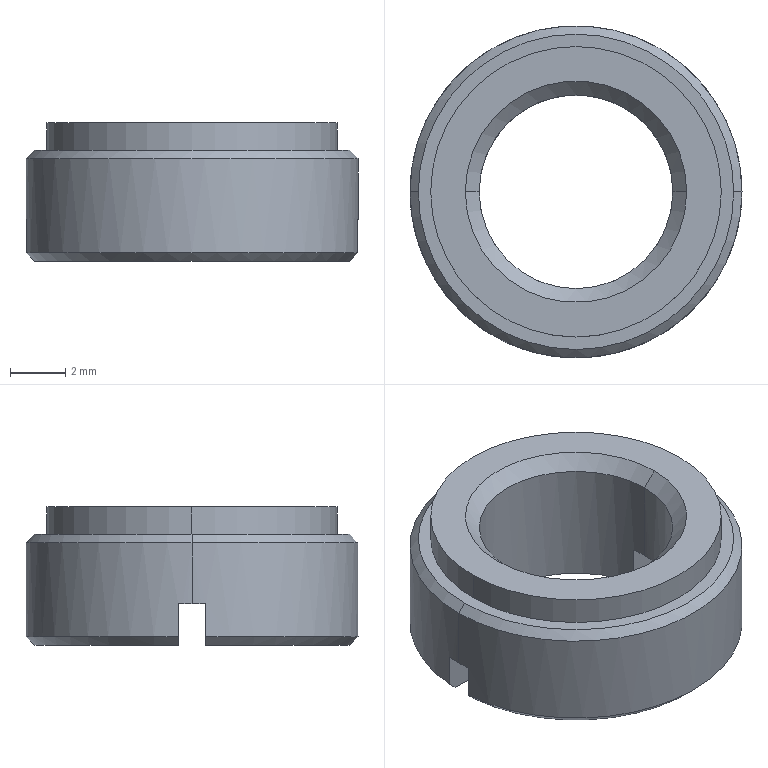Part | SolidWorks | features Chamfer 2, ICE 2, Extrusion 1 | 1 solid | 22 faces | box 12 x 12 x 5 mm | volume 332.916 mm3 | plane 10 | cone 6 | cylinder 6 | commonest cylinder face diameters 7 x2 10.5 x2 12 x2
STEP:
#1=CARTESIAN_POINT('',(5.7,0.,4.));
#2=VERTEX_POINT('',#1);
#3=CARTESIAN_POINT('',(-5.7,0.,4.));
#4=VERTEX_POINT('',#3);
#5=CARTESIAN_POINT('',(0.,0.,4.));
#6=DIRECTION('',(0.,0.,1.));
#7=DIRECTION('',(1.,0.,0.));
#8=AXIS2_PLACEMENT_3D('',#5,#6,#7);
#9=CIRCLE('',#8,5.7);
#10=EDGE_CURVE('',#2,#4,#9,.T.);
#11=ORIENTED_EDGE('',*,*,#10,.F.);
#12=CARTESIAN_POINT('',(6.,0.,3.7));
#13=VERTEX_POINT('',#12);
#14=CARTESIAN_POINT('',(5.7,0.,4.));
#15=DIRECTION('',(0.7071,0.,-0.7071));
#16=VECTOR('',#15,1000.);
#17=LINE('',#14,#16);
#18=EDGE_CURVE('',#2,#13,#17,.T.);
#19=ORIENTED_EDGE('',*,*,#18,.T.);
#20=CARTESIAN_POINT('',(-6.,0.,3.7));
#21=VERTEX_POINT('',#20);
#22=CARTESIAN_POINT('',(0.,0.,3.7));
#23=DIRECTION('',(0.,0.,-1.));
#24=DIRECTION('',(1.,0.,0.));
#25=AXIS2_PLACEMENT_3D('',#22,#23,#24);
#26=CIRCLE('',#25,6.);
#27=EDGE_CURVE('',#21,#13,#26,.T.);
#28=ORIENTED_EDGE('',*,*,#27,.F.);
#29=CARTESIAN_POINT('',(-5.7,0.,4.));
#30=DIRECTION('',(-0.7071,0.,-0.7071));
#31=VECTOR('',#30,1000.);
#32=LINE('',#29,#31);
#33=EDGE_CURVE('',#4,#21,#32,.T.);
#34=ORIENTED_EDGE('',*,*,#33,.F.);
#35=EDGE_LOOP('',(#11,#19,#28,#34));
#36=FACE_OUTER_BOUND('',#35,.T.);
#37=CARTESIAN_POINT('',(0.,0.,4.));
#38=DIRECTION('',(0.,0.,-1.));
#39=DIRECTION('',(-1.,0.,0.));
#40=AXIS2_PLACEMENT_3D('',#37,#38,#39);
#41=CONICAL_SURFACE('',#40,5.7,0.7854);
#42=ADVANCED_FACE('',(#36),#41,.T.);
#43=CARTESIAN_POINT('',(5.25,0.,4.));
#44=VERTEX_POINT('',#43);
#45=CARTESIAN_POINT('',(-5.25,0.,4.));
#46=VERTEX_POINT('',#45);
#47=CARTESIAN_POINT('',(0.,0.,4.));
#48=DIRECTION('',(0.,0.,1.));
#49=DIRECTION('',(1.,0.,0.));
#50=AXIS2_PLACEMENT_3D('',#47,#48,#49);
#51=CIRCLE('',#50,5.25);
#52=EDGE_CURVE('',#44,#46,#51,.T.);
#53=ORIENTED_EDGE('',*,*,#52,.T.);
#54=CARTESIAN_POINT('',(-5.25,0.,5.));
#55=VERTEX_POINT('',#54);
#56=CARTESIAN_POINT('',(-5.25,0.,4.));
#57=DIRECTION('',(0.,0.,1.));
#58=VECTOR('',#57,1000.);
#59=LINE('',#56,#58);
#60=EDGE_CURVE('',#46,#55,#59,.T.);
#61=ORIENTED_EDGE('',*,*,#60,.T.);
#62=CARTESIAN_POINT('',(5.25,0.,5.));
#63=VERTEX_POINT('',#62);
#64=CARTESIAN_POINT('',(0.,0.,5.));
#65=DIRECTION('',(0.,0.,1.));
#66=DIRECTION('',(1.,0.,0.));
#67=AXIS2_PLACEMENT_3D('',#64,#65,#66);
#68=CIRCLE('',#67,5.25);
#69=EDGE_CURVE('',#63,#55,#68,.T.);
#70=ORIENTED_EDGE('',*,*,#69,.F.);
#71=CARTESIAN_POINT('',(5.25,0.,4.));
#72=DIRECTION('',(0.,0.,1.));
#73=VECTOR('',#72,1000.);
#74=LINE('',#71,#73);
#75=EDGE_CURVE('',#44,#63,#74,.T.);
#76=ORIENTED_EDGE('',*,*,#75,.F.);
#77=EDGE_LOOP('',(#53,#61,#70,#76));
#78=FACE_OUTER_BOUND('',#77,.T.);
#79=CARTESIAN_POINT('',(0.,0.,4.));
#80=DIRECTION('',(0.,0.,1.));
#81=DIRECTION('',(1.,0.,0.));
#82=AXIS2_PLACEMENT_3D('',#79,#80,#81);
#83=CYLINDRICAL_SURFACE('',#82,5.25);
#84=ADVANCED_FACE('',(#78),#83,.T.);
#85=CARTESIAN_POINT('',(-3.5,0.,4.5));
#86=VERTEX_POINT('',#85);
#87=CARTESIAN_POINT('',(3.5,0.,4.5));
#88=VERTEX_POINT('',#87);
#89=CARTESIAN_POINT('',(0.,0.,4.5));
#90=DIRECTION('',(0.,0.,1.));
#91=DIRECTION('',(1.,0.,0.));
#92=AXIS2_PLACEMENT_3D('',#89,#90,#91);
#93=CIRCLE('',#92,3.5);
#94=EDGE_CURVE('',#86,#88,#93,.T.);
#95=ORIENTED_EDGE('',*,*,#94,.F.);
#96=CARTESIAN_POINT('',(-4.,0.,5.));
#97=VERTEX_POINT('',#96);
#98=CARTESIAN_POINT('',(-3.5,0.,4.5));
#99=DIRECTION('',(-0.7071,0.,0.7071));
#100=VECTOR('',#99,1000.);
#101=LINE('',#98,#100);
#102=EDGE_CURVE('',#86,#97,#101,.T.);
#103=ORIENTED_EDGE('',*,*,#102,.T.);
#104=CARTESIAN_POINT('',(4.,0.,5.));
#105=VERTEX_POINT('',#104);
#106=CARTESIAN_POINT('',(0.,0.,5.));
#107=DIRECTION('',(0.,0.,-1.));
#108=DIRECTION('',(1.,0.,0.));
#109=AXIS2_PLACEMENT_3D('',#106,#107,#108);
#110=CIRCLE('',#109,4.);
#111=EDGE_CURVE('',#105,#97,#110,.T.);
#112=ORIENTED_EDGE('',*,*,#111,.F.);
#113=CARTESIAN_POINT('',(3.5,0.,4.5));
#114=DIRECTION('',(0.7071,0.,0.7071));
#115=VECTOR('',#114,1000.);
#116=LINE('',#113,#115);
#117=EDGE_CURVE('',#88,#105,#116,.T.);
#118=ORIENTED_EDGE('',*,*,#117,.F.);
#119=EDGE_LOOP('',(#95,#103,#112,#118));
#120=FACE_OUTER_BOUND('',#119,.T.);
#121=CARTESIAN_POINT('',(0.,0.,4.5));
#122=DIRECTION('',(0.,0.,1.));
#123=DIRECTION('',(1.,0.,0.));
#124=AXIS2_PLACEMENT_3D('',#121,#122,#123);
#125=CONICAL_SURFACE('',#124,3.5,0.7854);
#126=ADVANCED_FACE('',(#120),#125,.F.);
#127=ORIENTED_EDGE('',*,*,#94,.T.);
#128=CARTESIAN_POINT('',(3.5,0.,1.5));
#129=VERTEX_POINT('',#128);
#130=CARTESIAN_POINT('',(3.5,0.,5.));
#131=DIRECTION('',(0.,0.,-1.));
#132=VECTOR('',#131,1000.);
#133=LINE('',#130,#132);
#134=EDGE_CURVE('',#88,#129,#133,.T.);
#135=ORIENTED_EDGE('',*,*,#134,.T.);
#136=CARTESIAN_POINT('',(3.464,-0.5,1.5));
#137=VERTEX_POINT('',#136);
#138=CARTESIAN_POINT('',(0.,0.,1.5));
#139=DIRECTION('',(0.,0.,-1.));
#140=DIRECTION('',(-1.,0.,0.));
#141=AXIS2_PLACEMENT_3D('',#138,#139,#140);
#142=CIRCLE('',#141,3.5);
#143=EDGE_CURVE('',#129,#137,#142,.T.);
#144=ORIENTED_EDGE('',*,*,#143,.T.);
#145=CARTESIAN_POINT('',(3.464,-0.5,0.));
#146=VERTEX_POINT('',#145);
#147=CARTESIAN_POINT('',(3.464,-0.5,5.));
#148=DIRECTION('',(0.,0.,1.));
#149=VECTOR('',#148,1000.);
#150=LINE('',#147,#149);
#151=EDGE_CURVE('',#146,#137,#150,.T.);
#152=ORIENTED_EDGE('',*,*,#151,.F.);
#153=CARTESIAN_POINT('',(-3.464,-0.5,0.));
#154=VERTEX_POINT('',#153);
#155=CARTESIAN_POINT('',(0.,0.,0.));
#156=DIRECTION('',(0.,0.,1.));
#157=DIRECTION('',(1.,0.,0.));
#158=AXIS2_PLACEMENT_3D('',#155,#156,#157);
#159=CIRCLE('',#158,3.5);
#160=EDGE_CURVE('',#154,#146,#159,.T.);
#161=ORIENTED_EDGE('',*,*,#160,.F.);
#162=CARTESIAN_POINT('',(-3.464,-0.5,1.5));
#163=VERTEX_POINT('',#162);
#164=CARTESIAN_POINT('',(-3.464,-0.5,5.));
#165=DIRECTION('',(0.,0.,-1.));
#166=VECTOR('',#165,1000.);
#167=LINE('',#164,#166);
#168=EDGE_CURVE('',#163,#154,#167,.T.);
#169=ORIENTED_EDGE('',*,*,#168,.F.);
#170=CARTESIAN_POINT('',(-3.5,0.,1.5));
#171=VERTEX_POINT('',#170);
#172=CARTESIAN_POINT('',(0.,0.,1.5));
#173=DIRECTION('',(0.,0.,-1.));
#174=DIRECTION('',(-1.,0.,0.));
#175=AXIS2_PLACEMENT_3D('',#172,#173,#174);
#176=CIRCLE('',#175,3.5);
#177=EDGE_CURVE('',#163,#171,#176,.T.);
#178=ORIENTED_EDGE('',*,*,#177,.T.);
#179=CARTESIAN_POINT('',(-3.5,0.,5.));
#180=DIRECTION('',(0.,0.,-1.));
#181=VECTOR('',#180,1000.);
#182=LINE('',#179,#181);
#183=EDGE_CURVE('',#86,#171,#182,.T.);
#184=ORIENTED_EDGE('',*,*,#183,.F.);
#185=EDGE_LOOP('',(#127,#135,#144,#152,#161,#169,#178,#184));
#186=FACE_OUTER_BOUND('',#185,.T.);
#187=CARTESIAN_POINT('',(0.,0.,5.));
#188=DIRECTION('',(0.,0.,-1.));
#189=DIRECTION('',(-1.,0.,0.));
#190=AXIS2_PLACEMENT_3D('',#187,#188,#189);
#191=CYLINDRICAL_SURFACE('',#190,3.5);
#192=ADVANCED_FACE('',(#186),#191,.F.);
#193=ORIENTED_EDGE('',*,*,#27,.T.);
#194=CARTESIAN_POINT('',(6.,0.,1.5));
#195=VERTEX_POINT('',#194);
#196=CARTESIAN_POINT('',(6.,0.,5.));
#197=DIRECTION('',(0.,0.,-1.));
#198=VECTOR('',#197,1000.);
#199=LINE('',#196,#198);
#200=EDGE_CURVE('',#13,#195,#199,.T.);
#201=ORIENTED_EDGE('',*,*,#200,.T.);
#202=CARTESIAN_POINT('',(5.979,0.5,1.5));
#203=VERTEX_POINT('',#202);
#204=CARTESIAN_POINT('',(0.,0.,1.5));
#205=DIRECTION('',(0.,0.,-1.));
#206=DIRECTION('',(-1.,0.,0.));
#207=AXIS2_PLACEMENT_3D('',#204,#205,#206);
#208=CIRCLE('',#207,6.);
#209=EDGE_CURVE('',#203,#195,#208,.T.);
#210=ORIENTED_EDGE('',*,*,#209,.F.);
#211=CARTESIAN_POINT('',(5.979,0.5,0.3));
#212=VERTEX_POINT('',#211);
#213=CARTESIAN_POINT('',(5.979,0.5,5.));
#214=DIRECTION('',(0.,0.,-1.));
#215=VECTOR('',#214,1000.);
#216=LINE('',#213,#215);
#217=EDGE_CURVE('',#203,#212,#216,.T.);
#218=ORIENTED_EDGE('',*,*,#217,.T.);
#219=CARTESIAN_POINT('',(-5.979,0.5,0.3));
#220=VERTEX_POINT('',#219);
#221=CARTESIAN_POINT('',(0.,0.,0.3));
#222=DIRECTION('',(0.,0.,1.));
#223=DIRECTION('',(1.,0.,0.));
#224=AXIS2_PLACEMENT_3D('',#221,#222,#223);
#225=CIRCLE('',#224,6.);
#226=EDGE_CURVE('',#212,#220,#225,.T.);
#227=ORIENTED_EDGE('',*,*,#226,.T.);
#228=CARTESIAN_POINT('',(-5.979,0.5,1.5));
#229=VERTEX_POINT('',#228);
#230=CARTESIAN_POINT('',(-5.979,0.5,5.));
#231=DIRECTION('',(0.,0.,1.));
#232=VECTOR('',#231,1000.);
#233=LINE('',#230,#232);
#234=EDGE_CURVE('',#220,#229,#233,.T.);
#235=ORIENTED_EDGE('',*,*,#234,.T.);
#236=CARTESIAN_POINT('',(-6.,0.,1.5));
#237=VERTEX_POINT('',#236);
#238=CARTESIAN_POINT('',(0.,0.,1.5));
#239=DIRECTION('',(0.,0.,-1.));
#240=DIRECTION('',(-1.,0.,0.));
#241=AXIS2_PLACEMENT_3D('',#238,#239,#240);
#242=CIRCLE('',#241,6.);
#243=EDGE_CURVE('',#237,#229,#242,.T.);
#244=ORIENTED_EDGE('',*,*,#243,.F.);
#245=CARTESIAN_POINT('',(-6.,0.,5.));
#246=DIRECTION('',(0.,0.,-1.));
#247=VECTOR('',#246,1000.);
#248=LINE('',#245,#247);
#249=EDGE_CURVE('',#21,#237,#248,.T.);
#250=ORIENTED_EDGE('',*,*,#249,.F.);
#251=EDGE_LOOP('',(#193,#201,#210,#218,#227,#235,#244,#250));
#252=FACE_OUTER_BOUND('',#251,.T.);
#253=CARTESIAN_POINT('',(0.,0.,5.));
#254=DIRECTION('',(0.,0.,-1.));
#255=DIRECTION('',(-1.,0.,0.));
#256=AXIS2_PLACEMENT_3D('',#253,#254,#255);
#257=CYLINDRICAL_SURFACE('',#256,6.);
#258=ADVANCED_FACE('',(#252),#257,.T.);
#259=ORIENTED_EDGE('',*,*,#111,.T.);
#260=CARTESIAN_POINT('',(0.,0.,5.));
#261=DIRECTION('',(0.,0.,-1.));
#262=DIRECTION('',(1.,0.,0.));
#263=AXIS2_PLACEMENT_3D('',#260,#261,#262);
#264=CIRCLE('',#263,4.);
#265=EDGE_CURVE('',#97,#105,#264,.T.);
#266=ORIENTED_EDGE('',*,*,#265,.T.);
#267=EDGE_LOOP('',(#259,#266));
#268=FACE_BOUND('',#267,.T.);
#269=ORIENTED_EDGE('',*,*,#69,.T.);
#270=CARTESIAN_POINT('',(0.,0.,5.));
#271=DIRECTION('',(0.,0.,1.));
#272=DIRECTION('',(1.,0.,0.));
#273=AXIS2_PLACEMENT_3D('',#270,#271,#272);
#274=CIRCLE('',#273,5.25);
#275=EDGE_CURVE('',#55,#63,#274,.T.);
#276=ORIENTED_EDGE('',*,*,#275,.T.);
#277=EDGE_LOOP('',(#269,#276));
#278=FACE_OUTER_BOUND('',#277,.T.);
#279=CARTESIAN_POINT('',(0.,0.,5.));
#280=DIRECTION('',(0.,0.,1.));
#281=DIRECTION('',(1.,0.,0.));
#282=AXIS2_PLACEMENT_3D('',#279,#280,#281);
#283=PLANE('',#282);
#284=ADVANCED_FACE('',(#268,#278),#283,.T.);
#285=ORIENTED_EDGE('',*,*,#200,.F.);
#286=CARTESIAN_POINT('',(0.,0.,3.7));
#287=DIRECTION('',(0.,0.,-1.));
#288=DIRECTION('',(1.,0.,0.));
#289=AXIS2_PLACEMENT_3D('',#286,#287,#288);
#290=CIRCLE('',#289,6.);
#291=EDGE_CURVE('',#13,#21,#290,.T.);
#292=ORIENTED_EDGE('',*,*,#291,.T.);
#293=ORIENTED_EDGE('',*,*,#249,.T.);
#294=CARTESIAN_POINT('',(-5.979,-0.5,1.5));
#295=VERTEX_POINT('',#294);
#296=CARTESIAN_POINT('',(0.,0.,1.5));
#297=DIRECTION('',(0.,0.,-1.));
#298=DIRECTION('',(-1.,0.,0.));
#299=AXIS2_PLACEMENT_3D('',#296,#297,#298);
#300=CIRCLE('',#299,6.);
#301=EDGE_CURVE('',#295,#237,#300,.T.);
#302=ORIENTED_EDGE('',*,*,#301,.F.);
#303=CARTESIAN_POINT('',(-5.979,-0.5,0.3));
#304=VERTEX_POINT('',#303);
#305=CARTESIAN_POINT('',(-5.979,-0.5,5.));
#306=DIRECTION('',(0.,0.,-1.));
#307=VECTOR('',#306,1000.);
#308=LINE('',#305,#307);
#309=EDGE_CURVE('',#295,#304,#308,.T.);
#310=ORIENTED_EDGE('',*,*,#309,.T.);
#311=CARTESIAN_POINT('',(5.979,-0.5,0.3));
#312=VERTEX_POINT('',#311);
#313=CARTESIAN_POINT('',(0.,0.,0.3));
#314=DIRECTION('',(0.,0.,1.));
#315=DIRECTION('',(1.,0.,0.));
#316=AXIS2_PLACEMENT_3D('',#313,#314,#315);
#317=CIRCLE('',#316,6.);
#318=EDGE_CURVE('',#304,#312,#317,.T.);
#319=ORIENTED_EDGE('',*,*,#318,.T.);
#320=CARTESIAN_POINT('',(5.979,-0.5,1.5));
#321=VERTEX_POINT('',#320);
#322=CARTESIAN_POINT('',(5.979,-0.5,5.));
#323=DIRECTION('',(0.,0.,1.));
#324=VECTOR('',#323,1000.);
#325=LINE('',#322,#324);
#326=EDGE_CURVE('',#312,#321,#325,.T.);
#327=ORIENTED_EDGE('',*,*,#326,.T.);
#328=CARTESIAN_POINT('',(0.,0.,1.5));
#329=DIRECTION('',(0.,0.,-1.));
#330=DIRECTION('',(-1.,0.,0.));
#331=AXIS2_PLACEMENT_3D('',#328,#329,#330);
#332=CIRCLE('',#331,6.);
#333=EDGE_CURVE('',#195,#321,#332,.T.);
#334=ORIENTED_EDGE('',*,*,#333,.F.);
#335=EDGE_LOOP('',(#285,#292,#293,#302,#310,#319,#327,#334));
#336=FACE_OUTER_BOUND('',#335,.T.);
#337=CARTESIAN_POINT('',(0.,0.,5.));
#338=DIRECTION('',(0.,0.,-1.));
#339=DIRECTION('',(-1.,0.,0.));
#340=AXIS2_PLACEMENT_3D('',#337,#338,#339);
#341=CYLINDRICAL_SURFACE('',#340,6.);
#342=ADVANCED_FACE('',(#336),#341,.T.);
#343=CARTESIAN_POINT('',(-5.678,0.5,0.));
#344=VERTEX_POINT('',#343);
#345=CARTESIAN_POINT('',(-3.464,0.5,0.));
#346=VERTEX_POINT('',#345);
#347=CARTESIAN_POINT('',(8.749,0.5,0.));
#348=DIRECTION('',(1.,0.,0.));
#349=VECTOR('',#348,1000.);
#350=LINE('',#347,#349);
#351=EDGE_CURVE('',#344,#346,#350,.T.);
#352=ORIENTED_EDGE('',*,*,#351,.F.);
#353=CARTESIAN_POINT('',(5.678,0.5,0.));
#354=VERTEX_POINT('',#353);
#355=CARTESIAN_POINT('',(0.,0.,0.));
#356=DIRECTION('',(0.,0.,-1.));
#357=DIRECTION('',(1.,0.,0.));
#358=AXIS2_PLACEMENT_3D('',#355,#356,#357);
#359=CIRCLE('',#358,5.7);
#360=EDGE_CURVE('',#344,#354,#359,.T.);
#361=ORIENTED_EDGE('',*,*,#360,.T.);
#362=CARTESIAN_POINT('',(3.464,0.5,0.));
#363=VERTEX_POINT('',#362);
#364=CARTESIAN_POINT('',(8.749,0.5,0.));
#365=DIRECTION('',(1.,0.,0.));
#366=VECTOR('',#365,1000.);
#367=LINE('',#364,#366);
#368=EDGE_CURVE('',#363,#354,#367,.T.);
#369=ORIENTED_EDGE('',*,*,#368,.F.);
#370=CARTESIAN_POINT('',(0.,0.,0.));
#371=DIRECTION('',(0.,0.,1.));
#372=DIRECTION('',(1.,0.,0.));
#373=AXIS2_PLACEMENT_3D('',#370,#371,#372);
#374=CIRCLE('',#373,3.5);
#375=EDGE_CURVE('',#363,#346,#374,.T.);
#376=ORIENTED_EDGE('',*,*,#375,.T.);
#377=EDGE_LOOP('',(#352,#361,#369,#376));
#378=FACE_OUTER_BOUND('',#377,.T.);
#379=CARTESIAN_POINT('',(0.,0.,0.));
#380=DIRECTION('',(0.,0.,1.));
#381=DIRECTION('',(1.,0.,0.));
#382=AXIS2_PLACEMENT_3D('',#379,#380,#381);
#383=PLANE('',#382);
#384=ADVANCED_FACE('',(#378),#383,.F.);
#385=CARTESIAN_POINT('',(5.678,-0.5,0.));
#386=VERTEX_POINT('',#385);
#387=CARTESIAN_POINT('',(8.749,-0.5,0.));
#388=DIRECTION('',(-1.,0.,0.));
#389=VECTOR('',#388,1000.);
#390=LINE('',#387,#389);
#391=EDGE_CURVE('',#386,#146,#390,.T.);
#392=ORIENTED_EDGE('',*,*,#391,.F.);
#393=CARTESIAN_POINT('',(-5.678,-0.5,0.));
#394=VERTEX_POINT('',#393);
#395=CARTESIAN_POINT('',(0.,0.,0.));
#396=DIRECTION('',(0.,0.,-1.));
#397=DIRECTION('',(1.,0.,0.));
#398=AXIS2_PLACEMENT_3D('',#395,#396,#397);
#399=CIRCLE('',#398,5.7);
#400=EDGE_CURVE('',#386,#394,#399,.T.);
#401=ORIENTED_EDGE('',*,*,#400,.T.);
#402=CARTESIAN_POINT('',(8.749,-0.5,0.));
#403=DIRECTION('',(-1.,0.,0.));
#404=VECTOR('',#403,1000.);
#405=LINE('',#402,#404);
#406=EDGE_CURVE('',#154,#394,#405,.T.);
#407=ORIENTED_EDGE('',*,*,#406,.F.);
#408=ORIENTED_EDGE('',*,*,#160,.T.);
#409=EDGE_LOOP('',(#392,#401,#407,#408));
#410=FACE_OUTER_BOUND('',#409,.T.);
#411=CARTESIAN_POINT('',(0.,0.,0.));
#412=DIRECTION('',(0.,0.,1.));
#413=DIRECTION('',(1.,0.,0.));
#414=AXIS2_PLACEMENT_3D('',#411,#412,#413);
#415=PLANE('',#414);
#416=ADVANCED_FACE('',(#410),#415,.F.);
#417=ORIENTED_EDGE('',*,*,#134,.F.);
#418=CARTESIAN_POINT('',(0.,0.,4.5));
#419=DIRECTION('',(0.,0.,1.));
#420=DIRECTION('',(1.,0.,0.));
#421=AXIS2_PLACEMENT_3D('',#418,#419,#420);
#422=CIRCLE('',#421,3.5);
#423=EDGE_CURVE('',#88,#86,#422,.T.);
#424=ORIENTED_EDGE('',*,*,#423,.T.);
#425=ORIENTED_EDGE('',*,*,#183,.T.);
#426=CARTESIAN_POINT('',(-3.464,0.5,1.5));
#427=VERTEX_POINT('',#426);
#428=CARTESIAN_POINT('',(0.,0.,1.5));
#429=DIRECTION('',(0.,0.,-1.));
#430=DIRECTION('',(-1.,0.,0.));
#431=AXIS2_PLACEMENT_3D('',#428,#429,#430);
#432=CIRCLE('',#431,3.5);
#433=EDGE_CURVE('',#171,#427,#432,.T.);
#434=ORIENTED_EDGE('',*,*,#433,.T.);
#435=CARTESIAN_POINT('',(-3.464,0.5,5.));
#436=DIRECTION('',(0.,0.,1.));
#437=VECTOR('',#436,1000.);
#438=LINE('',#435,#437);
#439=EDGE_CURVE('',#346,#427,#438,.T.);
#440=ORIENTED_EDGE('',*,*,#439,.F.);
#441=ORIENTED_EDGE('',*,*,#375,.F.);
#442=CARTESIAN_POINT('',(3.464,0.5,1.5));
#443=VERTEX_POINT('',#442);
#444=CARTESIAN_POINT('',(3.464,0.5,5.));
#445=DIRECTION('',(0.,0.,-1.));
#446=VECTOR('',#445,1000.);
#447=LINE('',#444,#446);
#448=EDGE_CURVE('',#443,#363,#447,.T.);
#449=ORIENTED_EDGE('',*,*,#448,.F.);
#450=CARTESIAN_POINT('',(0.,0.,1.5));
#451=DIRECTION('',(0.,0.,-1.));
#452=DIRECTION('',(-1.,0.,0.));
#453=AXIS2_PLACEMENT_3D('',#450,#451,#452);
#454=CIRCLE('',#453,3.5);
#455=EDGE_CURVE('',#443,#129,#454,.T.);
#456=ORIENTED_EDGE('',*,*,#455,.T.);
#457=EDGE_LOOP('',(#417,#424,#425,#434,#440,#441,#449,#456));
#458=FACE_OUTER_BOUND('',#457,.T.);
#459=CARTESIAN_POINT('',(0.,0.,5.));
#460=DIRECTION('',(0.,0.,-1.));
#461=DIRECTION('',(-1.,0.,0.));
#462=AXIS2_PLACEMENT_3D('',#459,#460,#461);
#463=CYLINDRICAL_SURFACE('',#462,3.5);
#464=ADVANCED_FACE('',(#458),#463,.F.);
#465=ORIENTED_EDGE('',*,*,#102,.F.);
#466=ORIENTED_EDGE('',*,*,#423,.F.);
#467=ORIENTED_EDGE('',*,*,#117,.T.);
#468=ORIENTED_EDGE('',*,*,#265,.F.);
#469=EDGE_LOOP('',(#465,#466,#467,#468));
#470=FACE_OUTER_BOUND('',#469,.T.);
#471=CARTESIAN_POINT('',(0.,0.,4.5));
#472=DIRECTION('',(0.,0.,1.));
#473=DIRECTION('',(1.,0.,0.));
#474=AXIS2_PLACEMENT_3D('',#471,#472,#473);
#475=CONICAL_SURFACE('',#474,3.5,0.7854);
#476=ADVANCED_FACE('',(#470),#475,.F.);
#477=ORIENTED_EDGE('',*,*,#301,.T.);
#478=ORIENTED_EDGE('',*,*,#243,.T.);
#479=CARTESIAN_POINT('',(8.749,0.5,1.5));
#480=DIRECTION('',(1.,0.,0.));
#481=VECTOR('',#480,1000.);
#482=LINE('',#479,#481);
#483=EDGE_CURVE('',#229,#427,#482,.T.);
#484=ORIENTED_EDGE('',*,*,#483,.T.);
#485=ORIENTED_EDGE('',*,*,#433,.F.);
#486=ORIENTED_EDGE('',*,*,#177,.F.);
#487=CARTESIAN_POINT('',(8.749,-0.5,1.5));
#488=DIRECTION('',(-1.,0.,0.));
#489=VECTOR('',#488,1000.);
#490=LINE('',#487,#489);
#491=EDGE_CURVE('',#163,#295,#490,.T.);
#492=ORIENTED_EDGE('',*,*,#491,.T.);
#493=EDGE_LOOP('',(#477,#478,#484,#485,#486,#492));
#494=FACE_OUTER_BOUND('',#493,.T.);
#495=CARTESIAN_POINT('',(8.749,-0.5,1.5));
#496=DIRECTION('',(0.,0.,-1.));
#497=DIRECTION('',(-1.,0.,0.));
#498=AXIS2_PLACEMENT_3D('',#495,#496,#497);
#499=PLANE('',#498);
#500=ADVANCED_FACE('',(#494),#499,.T.);
#501=ORIENTED_EDGE('',*,*,#406,.T.);
#502=CARTESIAN_POINT('',(-5.678,-0.5,0.));
#503=CARTESIAN_POINT('',(-5.778,-0.5,0.09999));
#504=CARTESIAN_POINT('',(-5.879,-0.5,0.2));
#505=CARTESIAN_POINT('',(-5.979,-0.5,0.3));
#506=B_SPLINE_CURVE_WITH_KNOTS('',3,(#502,#503,#504,#505),.UNSPECIFIED.,.F.,.F.,(4,4),(0.,0.000425),.UNSPECIFIED.);
#507=EDGE_CURVE('',#394,#304,#506,.T.);
#508=ORIENTED_EDGE('',*,*,#507,.T.);
#509=ORIENTED_EDGE('',*,*,#309,.F.);
#510=ORIENTED_EDGE('',*,*,#491,.F.);
#511=ORIENTED_EDGE('',*,*,#168,.T.);
#512=EDGE_LOOP('',(#501,#508,#509,#510,#511));
#513=FACE_OUTER_BOUND('',#512,.T.);
#514=CARTESIAN_POINT('',(8.749,-0.5,1.5));
#515=DIRECTION('',(0.,-1.,0.));
#516=DIRECTION('',(0.,0.,-1.));
#517=AXIS2_PLACEMENT_3D('',#514,#515,#516);
#518=PLANE('',#517);
#519=ADVANCED_FACE('',(#513),#518,.F.);
#520=ORIENTED_EDGE('',*,*,#234,.F.);
#521=CARTESIAN_POINT('',(-5.979,0.5,0.3));
#522=CARTESIAN_POINT('',(-5.879,0.5,0.2));
#523=CARTESIAN_POINT('',(-5.778,0.5,0.09999));
#524=CARTESIAN_POINT('',(-5.678,0.5,0.));
#525=B_SPLINE_CURVE_WITH_KNOTS('',3,(#521,#522,#523,#524),.UNSPECIFIED.,.F.,.F.,(4,4),(0.,0.000425),.UNSPECIFIED.);
#526=EDGE_CURVE('',#220,#344,#525,.T.);
#527=ORIENTED_EDGE('',*,*,#526,.T.);
#528=ORIENTED_EDGE('',*,*,#351,.T.);
#529=ORIENTED_EDGE('',*,*,#439,.T.);
#530=ORIENTED_EDGE('',*,*,#483,.F.);
#531=EDGE_LOOP('',(#520,#527,#528,#529,#530));
#532=FACE_OUTER_BOUND('',#531,.T.);
#533=CARTESIAN_POINT('',(8.749,0.5,1.5));
#534=DIRECTION('',(0.,1.,0.));
#535=DIRECTION('',(0.,0.,1.));
#536=AXIS2_PLACEMENT_3D('',#533,#534,#535);
#537=PLANE('',#536);
#538=ADVANCED_FACE('',(#532),#537,.F.);
#539=ORIENTED_EDGE('',*,*,#368,.T.);
#540=CARTESIAN_POINT('',(5.678,0.5,0.));
#541=CARTESIAN_POINT('',(5.778,0.5,0.09999));
#542=CARTESIAN_POINT('',(5.879,0.5,0.2));
#543=CARTESIAN_POINT('',(5.979,0.5,0.3));
#544=B_SPLINE_CURVE_WITH_KNOTS('',3,(#540,#541,#542,#543),.UNSPECIFIED.,.F.,.F.,(4,4),(0.,0.000425),.UNSPECIFIED.);
#545=EDGE_CURVE('',#354,#212,#544,.T.);
#546=ORIENTED_EDGE('',*,*,#545,.T.);
#547=ORIENTED_EDGE('',*,*,#217,.F.);
#548=CARTESIAN_POINT('',(8.749,0.5,1.5));
#549=DIRECTION('',(1.,0.,0.));
#550=VECTOR('',#549,1000.);
#551=LINE('',#548,#550);
#552=EDGE_CURVE('',#443,#203,#551,.T.);
#553=ORIENTED_EDGE('',*,*,#552,.F.);
#554=ORIENTED_EDGE('',*,*,#448,.T.);
#555=EDGE_LOOP('',(#539,#546,#547,#553,#554));
#556=FACE_OUTER_BOUND('',#555,.T.);
#557=CARTESIAN_POINT('',(8.749,0.5,1.5));
#558=DIRECTION('',(0.,1.,0.));
#559=DIRECTION('',(0.,0.,1.));
#560=AXIS2_PLACEMENT_3D('',#557,#558,#559);
#561=PLANE('',#560);
#562=ADVANCED_FACE('',(#556),#561,.F.);
#563=ORIENTED_EDGE('',*,*,#326,.F.);
#564=CARTESIAN_POINT('',(5.979,-0.5,0.3));
#565=CARTESIAN_POINT('',(5.879,-0.5,0.2));
#566=CARTESIAN_POINT('',(5.778,-0.5,0.09999));
#567=CARTESIAN_POINT('',(5.678,-0.5,0.));
#568=B_SPLINE_CURVE_WITH_KNOTS('',3,(#564,#565,#566,#567),.UNSPECIFIED.,.F.,.F.,(4,4),(0.,0.000425),.UNSPECIFIED.);
#569=EDGE_CURVE('',#312,#386,#568,.T.);
#570=ORIENTED_EDGE('',*,*,#569,.T.);
#571=ORIENTED_EDGE('',*,*,#391,.T.);
#572=ORIENTED_EDGE('',*,*,#151,.T.);
#573=CARTESIAN_POINT('',(8.749,-0.5,1.5));
#574=DIRECTION('',(-1.,0.,0.));
#575=VECTOR('',#574,1000.);
#576=LINE('',#573,#575);
#577=EDGE_CURVE('',#321,#137,#576,.T.);
#578=ORIENTED_EDGE('',*,*,#577,.F.);
#579=EDGE_LOOP('',(#563,#570,#571,#572,#578));
#580=FACE_OUTER_BOUND('',#579,.T.);
#581=CARTESIAN_POINT('',(8.749,-0.5,1.5));
#582=DIRECTION('',(0.,-1.,0.));
#583=DIRECTION('',(0.,0.,-1.));
#584=AXIS2_PLACEMENT_3D('',#581,#582,#583);
#585=PLANE('',#584);
#586=ADVANCED_FACE('',(#580),#585,.F.);
#587=ORIENTED_EDGE('',*,*,#209,.T.);
#588=ORIENTED_EDGE('',*,*,#333,.T.);
#589=ORIENTED_EDGE('',*,*,#577,.T.);
#590=ORIENTED_EDGE('',*,*,#143,.F.);
#591=ORIENTED_EDGE('',*,*,#455,.F.);
#592=ORIENTED_EDGE('',*,*,#552,.T.);
#593=EDGE_LOOP('',(#587,#588,#589,#590,#591,#592));
#594=FACE_OUTER_BOUND('',#593,.T.);
#595=CARTESIAN_POINT('',(8.749,-0.5,1.5));
#596=DIRECTION('',(0.,0.,-1.));
#597=DIRECTION('',(-1.,0.,0.));
#598=AXIS2_PLACEMENT_3D('',#595,#596,#597);
#599=PLANE('',#598);
#600=ADVANCED_FACE('',(#594),#599,.T.);
#601=CARTESIAN_POINT('',(0.,0.,4.));
#602=DIRECTION('',(0.,0.,1.));
#603=DIRECTION('',(1.,0.,0.));
#604=AXIS2_PLACEMENT_3D('',#601,#602,#603);
#605=CIRCLE('',#604,5.7);
#606=EDGE_CURVE('',#4,#2,#605,.T.);
#607=ORIENTED_EDGE('',*,*,#606,.T.);
#608=ORIENTED_EDGE('',*,*,#10,.T.);
#609=EDGE_LOOP('',(#607,#608));
#610=FACE_OUTER_BOUND('',#609,.T.);
#611=ORIENTED_EDGE('',*,*,#52,.F.);
#612=CARTESIAN_POINT('',(0.,0.,4.));
#613=DIRECTION('',(0.,0.,1.));
#614=DIRECTION('',(1.,0.,0.));
#615=AXIS2_PLACEMENT_3D('',#612,#613,#614);
#616=CIRCLE('',#615,5.25);
#617=EDGE_CURVE('',#46,#44,#616,.T.);
#618=ORIENTED_EDGE('',*,*,#617,.F.);
#619=EDGE_LOOP('',(#611,#618));
#620=FACE_BOUND('',#619,.T.);
#621=CARTESIAN_POINT('',(0.,0.,4.));
#622=DIRECTION('',(0.,0.,1.));
#623=DIRECTION('',(1.,0.,0.));
#624=AXIS2_PLACEMENT_3D('',#621,#622,#623);
#625=PLANE('',#624);
#626=ADVANCED_FACE('',(#610,#620),#625,.T.);
#627=ORIENTED_EDGE('',*,*,#60,.F.);
#628=ORIENTED_EDGE('',*,*,#617,.T.);
#629=ORIENTED_EDGE('',*,*,#75,.T.);
#630=ORIENTED_EDGE('',*,*,#275,.F.);
#631=EDGE_LOOP('',(#627,#628,#629,#630));
#632=FACE_OUTER_BOUND('',#631,.T.);
#633=CARTESIAN_POINT('',(0.,0.,4.));
#634=DIRECTION('',(0.,0.,1.));
#635=DIRECTION('',(1.,0.,0.));
#636=AXIS2_PLACEMENT_3D('',#633,#634,#635);
#637=CYLINDRICAL_SURFACE('',#636,5.25);
#638=ADVANCED_FACE('',(#632),#637,.T.);
#639=ORIENTED_EDGE('',*,*,#545,.F.);
#640=ORIENTED_EDGE('',*,*,#360,.F.);
#641=ORIENTED_EDGE('',*,*,#526,.F.);
#642=ORIENTED_EDGE('',*,*,#226,.F.);
#643=EDGE_LOOP('',(#639,#640,#641,#642));
#644=FACE_OUTER_BOUND('',#643,.T.);
#645=CARTESIAN_POINT('',(0.,0.,0.3));
#646=DIRECTION('',(0.,0.,1.));
#647=DIRECTION('',(1.,0.,0.));
#648=AXIS2_PLACEMENT_3D('',#645,#646,#647);
#649=CONICAL_SURFACE('',#648,6.,0.7854);
#650=ADVANCED_FACE('',(#644),#649,.T.);
#651=ORIENTED_EDGE('',*,*,#507,.F.);
#652=ORIENTED_EDGE('',*,*,#400,.F.);
#653=ORIENTED_EDGE('',*,*,#569,.F.);
#654=ORIENTED_EDGE('',*,*,#318,.F.);
#655=EDGE_LOOP('',(#651,#652,#653,#654));
#656=FACE_OUTER_BOUND('',#655,.T.);
#657=CARTESIAN_POINT('',(0.,0.,0.3));
#658=DIRECTION('',(0.,0.,1.));
#659=DIRECTION('',(1.,0.,0.));
#660=AXIS2_PLACEMENT_3D('',#657,#658,#659);
#661=CONICAL_SURFACE('',#660,6.,0.7854);
#662=ADVANCED_FACE('',(#656),#661,.T.);
#663=ORIENTED_EDGE('',*,*,#18,.F.);
#664=ORIENTED_EDGE('',*,*,#606,.F.);
#665=ORIENTED_EDGE('',*,*,#33,.T.);
#666=ORIENTED_EDGE('',*,*,#291,.F.);
#667=EDGE_LOOP('',(#663,#664,#665,#666));
#668=FACE_OUTER_BOUND('',#667,.T.);
#669=CARTESIAN_POINT('',(0.,0.,4.));
#670=DIRECTION('',(0.,0.,-1.));
#671=DIRECTION('',(-1.,0.,0.));
#672=AXIS2_PLACEMENT_3D('',#669,#670,#671);
#673=CONICAL_SURFACE('',#672,5.7,0.7854);
#674=ADVANCED_FACE('',(#668),#673,.T.);
#675=CLOSED_SHELL('',(#42,#84,#126,#192,#258,#284,#342,#384,#416,#464,#476,#500,#519,#538,#562,#586,#600,#626,#638,#650,#662,#674));
#676=MANIFOLD_SOLID_BREP('',#675);
#677=CARTESIAN_POINT('',(0.,0.,0.));
#678=DIRECTION('',(0.,0.,1.));
#679=DIRECTION('',(1.,0.,0.));
#680=AXIS2_PLACEMENT_3D('',#677,#678,#679);
#681=(LENGTH_UNIT()NAMED_UNIT(*)SI_UNIT(.MILLI.,.METRE.));
#682=UNCERTAINTY_MEASURE_WITH_UNIT(LENGTH_MEASURE(0.00001),#681,'','');
#683=(NAMED_UNIT(*)PLANE_ANGLE_UNIT()SI_UNIT($,.RADIAN.));
#684=(NAMED_UNIT(*)SI_UNIT($,.STERADIAN.)SOLID_ANGLE_UNIT());
#685=(GEOMETRIC_REPRESENTATION_CONTEXT(3)GLOBAL_UNCERTAINTY_ASSIGNED_CONTEXT((#682))GLOBAL_UNIT_ASSIGNED_CONTEXT((#681,#683,#684))REPRESENTATION_CONTEXT('',''));
#686=ADVANCED_BREP_SHAPE_REPRESENTATION('',(#676,#680),#685);